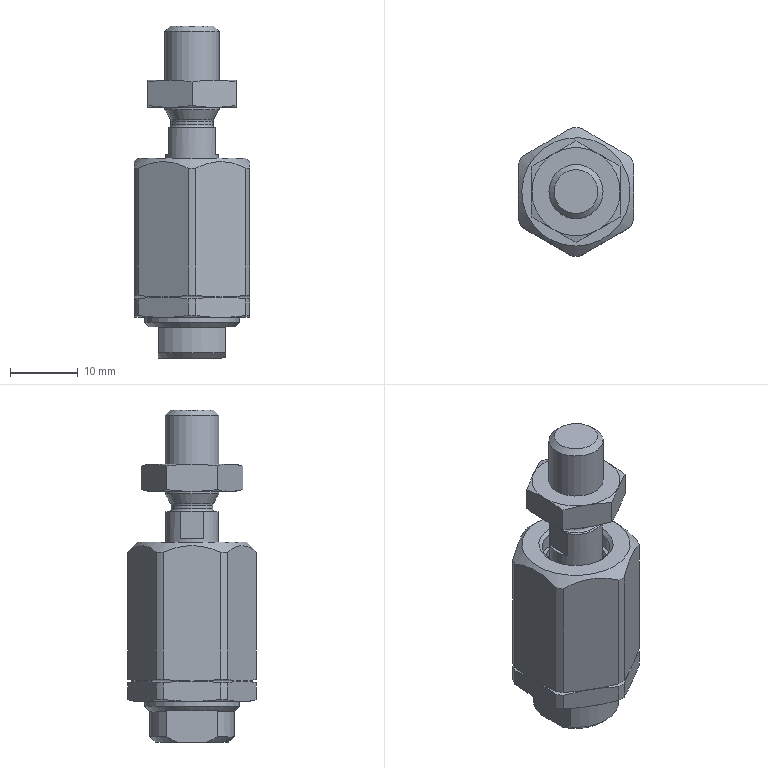Part | STEP file | 2062 FK-M8 | 7 solids | 126 faces | box 17 x 19 x 49 mm | volume 7068 mm3 | cone 47 | plane 44 | cylinder 29 | sphere 4 | torus 2 | commonest cylinder face diameters 19 x12 6.647 x2 9 x2 12.4 x2 12.5 x2 12.917 x2